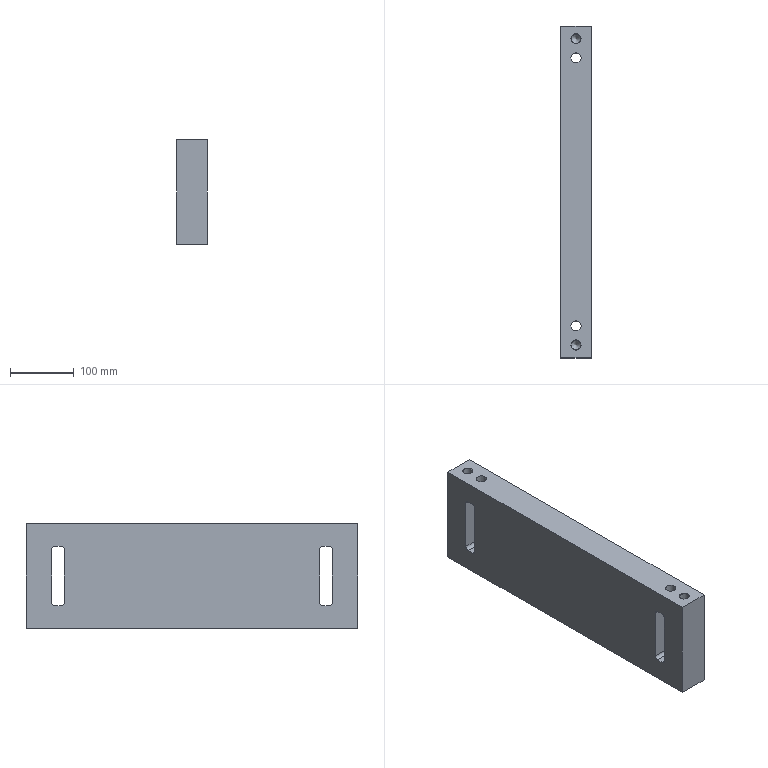Part | NX | features B2-1 2 | 1 solid | 42 faces | box 48 x 520 x 163 mm | volume 3822471 mm3 | plane 18 | cylinder 16 | cone 8 | commonest cylinder face diameters 10 x8 14.506 x4 16 x4
STEP:
#1=CARTESIAN_POINT('',(2312.849,-654.122,698.716));
#2=VERTEX_POINT('',#1);
#3=CARTESIAN_POINT('',(2312.849,-644.122,698.716));
#4=VERTEX_POINT('',#3);
#5=CARTESIAN_POINT('',(2319.094,-649.122,698.716));
#6=DIRECTION('',(0.,0.,1.));
#7=DIRECTION('',(1.,0.,0.));
#8=AXIS2_PLACEMENT_3D('',#5,#6,#7);
#9=CIRCLE('',#8,8.);
#10=EDGE_CURVE('',#2,#4,#9,.F.);
#11=ORIENTED_EDGE('',*,*,#10,.T.);
#12=CARTESIAN_POINT('',(2325.339,-644.122,698.716));
#13=VERTEX_POINT('',#12);
#14=CARTESIAN_POINT('',(2312.849,-644.122,698.716));
#15=CARTESIAN_POINT('',(2313.613,-643.167,698.716));
#16=CARTESIAN_POINT('',(2315.499,-641.68,698.187));
#17=CARTESIAN_POINT('',(2319.097,-640.842,697.481));
#18=CARTESIAN_POINT('',(2322.692,-641.683,698.188));
#19=CARTESIAN_POINT('',(2324.574,-643.166,698.716));
#20=CARTESIAN_POINT('',(2325.339,-644.122,698.716));
#21=B_SPLINE_CURVE_WITH_KNOTS('',3,(#14,#15,#16,#17,#18,#19,#20),.UNSPECIFIED.,.F.,.F.,(4,1,1,1,4),(0.,0.003599,0.007198,0.0108,0.0144),.UNSPECIFIED.);
#22=EDGE_CURVE('',#4,#13,#21,.T.);
#23=ORIENTED_EDGE('',*,*,#22,.T.);
#24=CARTESIAN_POINT('',(2325.339,-654.122,698.716));
#25=VERTEX_POINT('',#24);
#26=CARTESIAN_POINT('',(2319.094,-649.122,698.716));
#27=DIRECTION('',(0.,0.,1.));
#28=DIRECTION('',(1.,0.,0.));
#29=AXIS2_PLACEMENT_3D('',#26,#27,#28);
#30=CIRCLE('',#29,8.);
#31=EDGE_CURVE('',#13,#25,#30,.F.);
#32=ORIENTED_EDGE('',*,*,#31,.T.);
#33=CARTESIAN_POINT('',(2325.339,-654.122,698.716));
#34=CARTESIAN_POINT('',(2324.574,-655.077,698.716));
#35=CARTESIAN_POINT('',(2322.689,-656.564,698.187));
#36=CARTESIAN_POINT('',(2319.091,-657.402,697.481));
#37=CARTESIAN_POINT('',(2315.496,-656.562,698.188));
#38=CARTESIAN_POINT('',(2313.614,-655.078,698.716));
#39=CARTESIAN_POINT('',(2312.849,-654.122,698.716));
#40=B_SPLINE_CURVE_WITH_KNOTS('',3,(#33,#34,#35,#36,#37,#38,#39),.UNSPECIFIED.,.F.,.F.,(4,1,1,1,4),(0.,0.003599,0.007198,0.0108,0.0144),.UNSPECIFIED.);
#41=EDGE_CURVE('',#25,#2,#40,.T.);
#42=ORIENTED_EDGE('',*,*,#41,.T.);
#43=EDGE_LOOP('',(#11,#23,#32,#42));
#44=FACE_BOUND('',#43,.T.);
#45=CARTESIAN_POINT('',(2311.094,-649.122,733.716));
#46=VERTEX_POINT('',#45);
#47=CARTESIAN_POINT('',(2319.094,-649.122,733.716));
#48=DIRECTION('',(0.,0.,-1.));
#49=DIRECTION('',(-1.,0.,0.));
#50=AXIS2_PLACEMENT_3D('',#47,#48,#49);
#51=CIRCLE('',#50,8.);
#52=EDGE_CURVE('',#46,#46,#51,.T.);
#53=ORIENTED_EDGE('',*,*,#52,.F.);
#54=EDGE_LOOP('',(#53));
#55=FACE_BOUND('',#54,.T.);
#56=CARTESIAN_POINT('',(2319.094,-649.122,633.716));
#57=DIRECTION('',(0.,0.,1.));
#58=DIRECTION('',(1.,0.,0.));
#59=AXIS2_PLACEMENT_3D('',#56,#57,#58);
#60=CYLINDRICAL_SURFACE('',#59,8.);
#61=ADVANCED_FACE('',(#44,#55),#60,.F.);
#62=CARTESIAN_POINT('',(2312.849,-1074.122,698.716));
#63=VERTEX_POINT('',#62);
#64=CARTESIAN_POINT('',(2312.849,-1064.122,698.716));
#65=VERTEX_POINT('',#64);
#66=CARTESIAN_POINT('',(2319.094,-1069.122,698.716));
#67=DIRECTION('',(0.,0.,1.));
#68=DIRECTION('',(1.,0.,0.));
#69=AXIS2_PLACEMENT_3D('',#66,#67,#68);
#70=CIRCLE('',#69,8.);
#71=EDGE_CURVE('',#63,#65,#70,.F.);
#72=ORIENTED_EDGE('',*,*,#71,.T.);
#73=CARTESIAN_POINT('',(2325.339,-1064.122,698.716));
#74=VERTEX_POINT('',#73);
#75=CARTESIAN_POINT('',(2312.849,-1064.122,698.716));
#76=CARTESIAN_POINT('',(2313.613,-1063.167,698.716));
#77=CARTESIAN_POINT('',(2315.499,-1061.68,698.187));
#78=CARTESIAN_POINT('',(2319.097,-1060.842,697.481));
#79=CARTESIAN_POINT('',(2322.692,-1061.683,698.188));
#80=CARTESIAN_POINT('',(2324.574,-1063.166,698.716));
#81=CARTESIAN_POINT('',(2325.339,-1064.122,698.716));
#82=B_SPLINE_CURVE_WITH_KNOTS('',3,(#75,#76,#77,#78,#79,#80,#81),.UNSPECIFIED.,.F.,.F.,(4,1,1,1,4),(0.,0.003599,0.007198,0.0108,0.0144),.UNSPECIFIED.);
#83=EDGE_CURVE('',#65,#74,#82,.T.);
#84=ORIENTED_EDGE('',*,*,#83,.T.);
#85=CARTESIAN_POINT('',(2325.339,-1074.122,698.716));
#86=VERTEX_POINT('',#85);
#87=CARTESIAN_POINT('',(2319.094,-1069.122,698.716));
#88=DIRECTION('',(0.,0.,1.));
#89=DIRECTION('',(1.,0.,0.));
#90=AXIS2_PLACEMENT_3D('',#87,#88,#89);
#91=CIRCLE('',#90,8.);
#92=EDGE_CURVE('',#74,#86,#91,.F.);
#93=ORIENTED_EDGE('',*,*,#92,.T.);
#94=CARTESIAN_POINT('',(2325.339,-1074.122,698.716));
#95=CARTESIAN_POINT('',(2324.574,-1075.077,698.716));
#96=CARTESIAN_POINT('',(2322.689,-1076.564,698.187));
#97=CARTESIAN_POINT('',(2319.091,-1077.402,697.481));
#98=CARTESIAN_POINT('',(2315.496,-1076.562,698.188));
#99=CARTESIAN_POINT('',(2313.614,-1075.078,698.716));
#100=CARTESIAN_POINT('',(2312.849,-1074.122,698.716));
#101=B_SPLINE_CURVE_WITH_KNOTS('',3,(#94,#95,#96,#97,#98,#99,#100),.UNSPECIFIED.,.F.,.F.,(4,1,1,1,4),(0.,0.003599,0.007198,0.0108,0.0144),.UNSPECIFIED.);
#102=EDGE_CURVE('',#86,#63,#101,.T.);
#103=ORIENTED_EDGE('',*,*,#102,.T.);
#104=EDGE_LOOP('',(#72,#84,#93,#103));
#105=FACE_BOUND('',#104,.T.);
#106=CARTESIAN_POINT('',(2311.094,-1069.122,733.716));
#107=VERTEX_POINT('',#106);
#108=CARTESIAN_POINT('',(2319.094,-1069.122,733.716));
#109=DIRECTION('',(0.,0.,-1.));
#110=DIRECTION('',(-1.,0.,0.));
#111=AXIS2_PLACEMENT_3D('',#108,#109,#110);
#112=CIRCLE('',#111,8.);
#113=EDGE_CURVE('',#107,#107,#112,.T.);
#114=ORIENTED_EDGE('',*,*,#113,.F.);
#115=EDGE_LOOP('',(#114));
#116=FACE_BOUND('',#115,.T.);
#117=CARTESIAN_POINT('',(2319.094,-1069.122,633.716));
#118=DIRECTION('',(0.,0.,1.));
#119=DIRECTION('',(1.,0.,0.));
#120=AXIS2_PLACEMENT_3D('',#117,#118,#119);
#121=CYLINDRICAL_SURFACE('',#120,8.);
#122=ADVANCED_FACE('',(#105,#116),#121,.F.);
#123=CARTESIAN_POINT('',(2295.094,-639.122,610.716));
#124=VERTEX_POINT('',#123);
#125=CARTESIAN_POINT('',(2295.094,-639.122,693.716));
#126=VERTEX_POINT('',#125);
#127=CARTESIAN_POINT('',(2295.094,-639.122,600.716));
#128=DIRECTION('',(0.,0.,1.));
#129=VECTOR('',#128,1000.);
#130=LINE('',#127,#129);
#131=EDGE_CURVE('',#124,#126,#130,.T.);
#132=ORIENTED_EDGE('',*,*,#131,.T.);
#133=CARTESIAN_POINT('',(2295.094,-644.122,698.716));
#134=VERTEX_POINT('',#133);
#135=CARTESIAN_POINT('',(2295.094,-644.122,693.716));
#136=DIRECTION('',(1.,0.,0.));
#137=DIRECTION('',(0.,0.,-1.));
#138=AXIS2_PLACEMENT_3D('',#135,#136,#137);
#139=CIRCLE('',#138,5.);
#140=EDGE_CURVE('',#126,#134,#139,.T.);
#141=ORIENTED_EDGE('',*,*,#140,.T.);
#142=CARTESIAN_POINT('',(2295.094,-654.122,698.716));
#143=VERTEX_POINT('',#142);
#144=CARTESIAN_POINT('',(2295.094,-599.122,698.716));
#145=DIRECTION('',(0.,-1.,0.));
#146=VECTOR('',#145,1000.);
#147=LINE('',#144,#146);
#148=EDGE_CURVE('',#134,#143,#147,.T.);
#149=ORIENTED_EDGE('',*,*,#148,.T.);
#150=CARTESIAN_POINT('',(2295.094,-659.122,693.716));
#151=VERTEX_POINT('',#150);
#152=CARTESIAN_POINT('',(2295.094,-654.122,693.716));
#153=DIRECTION('',(1.,0.,0.));
#154=DIRECTION('',(0.,0.,-1.));
#155=AXIS2_PLACEMENT_3D('',#152,#153,#154);
#156=CIRCLE('',#155,5.);
#157=EDGE_CURVE('',#143,#151,#156,.T.);
#158=ORIENTED_EDGE('',*,*,#157,.T.);
#159=CARTESIAN_POINT('',(2295.094,-659.122,610.716));
#160=VERTEX_POINT('',#159);
#161=CARTESIAN_POINT('',(2295.094,-659.122,600.716));
#162=DIRECTION('',(0.,0.,-1.));
#163=VECTOR('',#162,1000.);
#164=LINE('',#161,#163);
#165=EDGE_CURVE('',#151,#160,#164,.T.);
#166=ORIENTED_EDGE('',*,*,#165,.T.);
#167=CARTESIAN_POINT('',(2295.094,-654.122,605.716));
#168=VERTEX_POINT('',#167);
#169=CARTESIAN_POINT('',(2295.094,-654.122,610.716));
#170=DIRECTION('',(1.,0.,0.));
#171=DIRECTION('',(0.,0.,-1.));
#172=AXIS2_PLACEMENT_3D('',#169,#170,#171);
#173=CIRCLE('',#172,5.);
#174=EDGE_CURVE('',#160,#168,#173,.T.);
#175=ORIENTED_EDGE('',*,*,#174,.T.);
#176=CARTESIAN_POINT('',(2295.094,-644.122,605.716));
#177=VERTEX_POINT('',#176);
#178=CARTESIAN_POINT('',(2295.094,-599.122,605.716));
#179=DIRECTION('',(0.,1.,0.));
#180=VECTOR('',#179,1000.);
#181=LINE('',#178,#180);
#182=EDGE_CURVE('',#168,#177,#181,.T.);
#183=ORIENTED_EDGE('',*,*,#182,.T.);
#184=CARTESIAN_POINT('',(2295.094,-644.122,610.716));
#185=DIRECTION('',(1.,0.,0.));
#186=DIRECTION('',(0.,0.,-1.));
#187=AXIS2_PLACEMENT_3D('',#184,#185,#186);
#188=CIRCLE('',#187,5.);
#189=EDGE_CURVE('',#177,#124,#188,.T.);
#190=ORIENTED_EDGE('',*,*,#189,.T.);
#191=EDGE_LOOP('',(#132,#141,#149,#158,#166,#175,#183,#190));
#192=FACE_BOUND('',#191,.T.);
#193=CARTESIAN_POINT('',(2295.094,-1059.122,610.716));
#194=VERTEX_POINT('',#193);
#195=CARTESIAN_POINT('',(2295.094,-1059.122,693.716));
#196=VERTEX_POINT('',#195);
#197=CARTESIAN_POINT('',(2295.094,-1059.122,600.716));
#198=DIRECTION('',(0.,0.,1.));
#199=VECTOR('',#198,1000.);
#200=LINE('',#197,#199);
#201=EDGE_CURVE('',#194,#196,#200,.T.);
#202=ORIENTED_EDGE('',*,*,#201,.T.);
#203=CARTESIAN_POINT('',(2295.094,-1064.122,698.716));
#204=VERTEX_POINT('',#203);
#205=CARTESIAN_POINT('',(2295.094,-1064.122,693.716));
#206=DIRECTION('',(1.,0.,0.));
#207=DIRECTION('',(0.,0.,-1.));
#208=AXIS2_PLACEMENT_3D('',#205,#206,#207);
#209=CIRCLE('',#208,5.);
#210=EDGE_CURVE('',#196,#204,#209,.T.);
#211=ORIENTED_EDGE('',*,*,#210,.T.);
#212=CARTESIAN_POINT('',(2295.094,-1074.122,698.716));
#213=VERTEX_POINT('',#212);
#214=CARTESIAN_POINT('',(2295.094,-599.122,698.716));
#215=DIRECTION('',(0.,-1.,0.));
#216=VECTOR('',#215,1000.);
#217=LINE('',#214,#216);
#218=EDGE_CURVE('',#204,#213,#217,.T.);
#219=ORIENTED_EDGE('',*,*,#218,.T.);
#220=CARTESIAN_POINT('',(2295.094,-1079.122,693.716));
#221=VERTEX_POINT('',#220);
#222=CARTESIAN_POINT('',(2295.094,-1074.122,693.716));
#223=DIRECTION('',(1.,0.,0.));
#224=DIRECTION('',(0.,0.,-1.));
#225=AXIS2_PLACEMENT_3D('',#222,#223,#224);
#226=CIRCLE('',#225,5.);
#227=EDGE_CURVE('',#213,#221,#226,.T.);
#228=ORIENTED_EDGE('',*,*,#227,.T.);
#229=CARTESIAN_POINT('',(2295.094,-1079.122,610.716));
#230=VERTEX_POINT('',#229);
#231=CARTESIAN_POINT('',(2295.094,-1079.122,600.716));
#232=DIRECTION('',(0.,0.,-1.));
#233=VECTOR('',#232,1000.);
#234=LINE('',#231,#233);
#235=EDGE_CURVE('',#221,#230,#234,.T.);
#236=ORIENTED_EDGE('',*,*,#235,.T.);
#237=CARTESIAN_POINT('',(2295.094,-1074.122,605.716));
#238=VERTEX_POINT('',#237);
#239=CARTESIAN_POINT('',(2295.094,-1074.122,610.716));
#240=DIRECTION('',(1.,0.,0.));
#241=DIRECTION('',(0.,0.,-1.));
#242=AXIS2_PLACEMENT_3D('',#239,#240,#241);
#243=CIRCLE('',#242,5.);
#244=EDGE_CURVE('',#230,#238,#243,.T.);
#245=ORIENTED_EDGE('',*,*,#244,.T.);
#246=CARTESIAN_POINT('',(2295.094,-1064.122,605.716));
#247=VERTEX_POINT('',#246);
#248=CARTESIAN_POINT('',(2295.094,-599.122,605.716));
#249=DIRECTION('',(0.,1.,0.));
#250=VECTOR('',#249,1000.);
#251=LINE('',#248,#250);
#252=EDGE_CURVE('',#238,#247,#251,.T.);
#253=ORIENTED_EDGE('',*,*,#252,.T.);
#254=CARTESIAN_POINT('',(2295.094,-1064.122,610.716));
#255=DIRECTION('',(1.,0.,0.));
#256=DIRECTION('',(0.,0.,-1.));
#257=AXIS2_PLACEMENT_3D('',#254,#255,#256);
#258=CIRCLE('',#257,5.);
#259=EDGE_CURVE('',#247,#194,#258,.T.);
#260=ORIENTED_EDGE('',*,*,#259,.T.);
#261=EDGE_LOOP('',(#202,#211,#219,#228,#236,#245,#253,#260));
#262=FACE_BOUND('',#261,.T.);
#263=CARTESIAN_POINT('',(2295.094,-599.122,733.716));
#264=VERTEX_POINT('',#263);
#265=CARTESIAN_POINT('',(2295.094,-1119.122,733.716));
#266=VERTEX_POINT('',#265);
#267=CARTESIAN_POINT('',(2295.094,-599.122,733.716));
#268=DIRECTION('',(0.,-1.,0.));
#269=VECTOR('',#268,1000.);
#270=LINE('',#267,#269);
#271=EDGE_CURVE('',#264,#266,#270,.T.);
#272=ORIENTED_EDGE('',*,*,#271,.F.);
#273=CARTESIAN_POINT('',(2295.094,-599.122,570.716));
#274=VERTEX_POINT('',#273);
#275=CARTESIAN_POINT('',(2295.094,-599.122,600.716));
#276=DIRECTION('',(0.,0.,1.));
#277=VECTOR('',#276,1000.);
#278=LINE('',#275,#277);
#279=EDGE_CURVE('',#274,#264,#278,.T.);
#280=ORIENTED_EDGE('',*,*,#279,.F.);
#281=CARTESIAN_POINT('',(2295.094,-1119.122,570.716));
#282=VERTEX_POINT('',#281);
#283=CARTESIAN_POINT('',(2295.094,-599.122,570.716));
#284=DIRECTION('',(0.,-1.,0.));
#285=VECTOR('',#284,1000.);
#286=LINE('',#283,#285);
#287=EDGE_CURVE('',#274,#282,#286,.T.);
#288=ORIENTED_EDGE('',*,*,#287,.T.);
#289=CARTESIAN_POINT('',(2295.094,-1119.122,600.716));
#290=DIRECTION('',(0.,0.,1.));
#291=VECTOR('',#290,1000.);
#292=LINE('',#289,#291);
#293=EDGE_CURVE('',#282,#266,#292,.T.);
#294=ORIENTED_EDGE('',*,*,#293,.T.);
#295=EDGE_LOOP('',(#272,#280,#288,#294));
#296=FACE_BOUND('',#295,.T.);
#297=CARTESIAN_POINT('',(2295.094,-599.122,600.716));
#298=DIRECTION('',(1.,0.,0.));
#299=DIRECTION('',(0.,0.,1.));
#300=AXIS2_PLACEMENT_3D('',#297,#298,#299);
#301=PLANE('',#300);
#302=ADVANCED_FACE('',(#192,#262,#296),#301,.F.);
#303=CARTESIAN_POINT('',(2311.094,-649.122,570.716));
#304=VERTEX_POINT('',#303);
#305=CARTESIAN_POINT('',(2319.094,-649.122,570.716));
#306=DIRECTION('',(0.,0.,-1.));
#307=DIRECTION('',(-1.,0.,0.));
#308=AXIS2_PLACEMENT_3D('',#305,#306,#307);
#309=CIRCLE('',#308,8.);
#310=EDGE_CURVE('',#304,#304,#309,.T.);
#311=ORIENTED_EDGE('',*,*,#310,.F.);
#312=EDGE_LOOP('',(#311));
#313=FACE_BOUND('',#312,.T.);
#314=CARTESIAN_POINT('',(2311.094,-1069.122,570.716));
#315=VERTEX_POINT('',#314);
#316=CARTESIAN_POINT('',(2319.094,-1069.122,570.716));
#317=DIRECTION('',(0.,0.,-1.));
#318=DIRECTION('',(-1.,0.,0.));
#319=AXIS2_PLACEMENT_3D('',#316,#317,#318);
#320=CIRCLE('',#319,8.);
#321=EDGE_CURVE('',#315,#315,#320,.T.);
#322=ORIENTED_EDGE('',*,*,#321,.F.);
#323=EDGE_LOOP('',(#322));
#324=FACE_BOUND('',#323,.T.);
#325=CARTESIAN_POINT('',(2311.094,-679.122,570.716));
#326=VERTEX_POINT('',#325);
#327=CARTESIAN_POINT('',(2319.094,-679.122,570.716));
#328=DIRECTION('',(0.,0.,-1.));
#329=DIRECTION('',(-1.,0.,0.));
#330=AXIS2_PLACEMENT_3D('',#327,#328,#329);
#331=CIRCLE('',#330,8.);
#332=EDGE_CURVE('',#326,#326,#331,.T.);
#333=ORIENTED_EDGE('',*,*,#332,.F.);
#334=EDGE_LOOP('',(#333));
#335=FACE_BOUND('',#334,.T.);
#336=CARTESIAN_POINT('',(2311.094,-1039.122,570.716));
#337=VERTEX_POINT('',#336);
#338=CARTESIAN_POINT('',(2319.094,-1039.122,570.716));
#339=DIRECTION('',(0.,0.,-1.));
#340=DIRECTION('',(-1.,0.,0.));
#341=AXIS2_PLACEMENT_3D('',#338,#339,#340);
#342=CIRCLE('',#341,8.);
#343=EDGE_CURVE('',#337,#337,#342,.T.);
#344=ORIENTED_EDGE('',*,*,#343,.F.);
#345=EDGE_LOOP('',(#344));
#346=FACE_BOUND('',#345,.T.);
#347=CARTESIAN_POINT('',(2343.094,-599.122,570.716));
#348=VERTEX_POINT('',#347);
#349=CARTESIAN_POINT('',(2343.094,-1119.122,570.716));
#350=VERTEX_POINT('',#349);
#351=CARTESIAN_POINT('',(2343.094,0.,570.716));
#352=DIRECTION('',(0.,-1.,0.));
#353=VECTOR('',#352,1000.);
#354=LINE('',#351,#353);
#355=EDGE_CURVE('',#348,#350,#354,.T.);
#356=ORIENTED_EDGE('',*,*,#355,.T.);
#357=CARTESIAN_POINT('',(2295.094,-1119.122,570.716));
#358=DIRECTION('',(1.,0.,0.));
#359=VECTOR('',#358,1000.);
#360=LINE('',#357,#359);
#361=EDGE_CURVE('',#282,#350,#360,.T.);
#362=ORIENTED_EDGE('',*,*,#361,.F.);
#363=ORIENTED_EDGE('',*,*,#287,.F.);
#364=CARTESIAN_POINT('',(4420.094,-599.122,570.716));
#365=DIRECTION('',(-1.,0.,0.));
#366=VECTOR('',#365,1000.);
#367=LINE('',#364,#366);
#368=EDGE_CURVE('',#348,#274,#367,.T.);
#369=ORIENTED_EDGE('',*,*,#368,.F.);
#370=EDGE_LOOP('',(#356,#362,#363,#369));
#371=FACE_BOUND('',#370,.T.);
#372=CARTESIAN_POINT('',(6675.188,0.,570.716));
#373=DIRECTION('',(0.,0.,-1.));
#374=DIRECTION('',(1.,0.,0.));
#375=AXIS2_PLACEMENT_3D('',#372,#373,#374);
#376=PLANE('',#375);
#377=ADVANCED_FACE('',(#313,#324,#335,#346,#371),#376,.T.);
#378=ORIENTED_EDGE('',*,*,#52,.T.);
#379=EDGE_LOOP('',(#378));
#380=FACE_BOUND('',#379,.T.);
#381=ORIENTED_EDGE('',*,*,#113,.T.);
#382=EDGE_LOOP('',(#381));
#383=FACE_BOUND('',#382,.T.);
#384=CARTESIAN_POINT('',(2327.094,-619.122,733.716));
#385=VERTEX_POINT('',#384);
#386=CARTESIAN_POINT('',(2319.094,-619.122,733.716));
#387=DIRECTION('',(0.,0.,1.));
#388=DIRECTION('',(1.,0.,0.));
#389=AXIS2_PLACEMENT_3D('',#386,#387,#388);
#390=CIRCLE('',#389,8.);
#391=EDGE_CURVE('',#385,#385,#390,.T.);
#392=ORIENTED_EDGE('',*,*,#391,.F.);
#393=EDGE_LOOP('',(#392));
#394=FACE_BOUND('',#393,.T.);
#395=CARTESIAN_POINT('',(2327.094,-1099.122,733.716));
#396=VERTEX_POINT('',#395);
#397=CARTESIAN_POINT('',(2319.094,-1099.122,733.716));
#398=DIRECTION('',(0.,0.,1.));
#399=DIRECTION('',(1.,0.,0.));
#400=AXIS2_PLACEMENT_3D('',#397,#398,#399);
#401=CIRCLE('',#400,8.);
#402=EDGE_CURVE('',#396,#396,#401,.T.);
#403=ORIENTED_EDGE('',*,*,#402,.F.);
#404=EDGE_LOOP('',(#403));
#405=FACE_BOUND('',#404,.T.);
#406=CARTESIAN_POINT('',(2343.094,-599.122,733.716));
#407=VERTEX_POINT('',#406);
#408=CARTESIAN_POINT('',(4420.094,-599.122,733.716));
#409=DIRECTION('',(-1.,0.,0.));
#410=VECTOR('',#409,1000.);
#411=LINE('',#408,#410);
#412=EDGE_CURVE('',#407,#264,#411,.T.);
#413=ORIENTED_EDGE('',*,*,#412,.T.);
#414=ORIENTED_EDGE('',*,*,#271,.T.);
#415=CARTESIAN_POINT('',(2343.094,-1119.122,733.716));
#416=VERTEX_POINT('',#415);
#417=CARTESIAN_POINT('',(2295.094,-1119.122,733.716));
#418=DIRECTION('',(1.,0.,0.));
#419=VECTOR('',#418,1000.);
#420=LINE('',#417,#419);
#421=EDGE_CURVE('',#266,#416,#420,.T.);
#422=ORIENTED_EDGE('',*,*,#421,.T.);
#423=CARTESIAN_POINT('',(2343.094,-859.122,733.716));
#424=DIRECTION('',(0.,1.,0.));
#425=VECTOR('',#424,1000.);
#426=LINE('',#423,#425);
#427=EDGE_CURVE('',#416,#407,#426,.T.);
#428=ORIENTED_EDGE('',*,*,#427,.T.);
#429=EDGE_LOOP('',(#413,#414,#422,#428));
#430=FACE_BOUND('',#429,.T.);
#431=CARTESIAN_POINT('',(6675.188,0.,733.716));
#432=DIRECTION('',(0.,0.,-1.));
#433=DIRECTION('',(1.,0.,0.));
#434=AXIS2_PLACEMENT_3D('',#431,#432,#433);
#435=PLANE('',#434);
#436=ADVANCED_FACE('',(#380,#383,#394,#405,#430),#435,.F.);
#437=ORIENTED_EDGE('',*,*,#421,.F.);
#438=ORIENTED_EDGE('',*,*,#293,.F.);
#439=ORIENTED_EDGE('',*,*,#361,.T.);
#440=CARTESIAN_POINT('',(2343.094,-1119.122,600.716));
#441=DIRECTION('',(0.,0.,-1.));
#442=VECTOR('',#441,1000.);
#443=LINE('',#440,#442);
#444=EDGE_CURVE('',#416,#350,#443,.T.);
#445=ORIENTED_EDGE('',*,*,#444,.F.);
#446=EDGE_LOOP('',(#437,#438,#439,#445));
#447=FACE_BOUND('',#446,.T.);
#448=CARTESIAN_POINT('',(2295.094,-1119.122,600.716));
#449=DIRECTION('',(0.,1.,0.));
#450=DIRECTION('',(1.,0.,0.));
#451=AXIS2_PLACEMENT_3D('',#448,#449,#450);
#452=PLANE('',#451);
#453=ADVANCED_FACE('',(#447),#452,.F.);
#454=ORIENTED_EDGE('',*,*,#368,.T.);
#455=ORIENTED_EDGE('',*,*,#279,.T.);
#456=ORIENTED_EDGE('',*,*,#412,.F.);
#457=CARTESIAN_POINT('',(2343.094,-599.122,600.716));
#458=DIRECTION('',(0.,0.,1.));
#459=VECTOR('',#458,1000.);
#460=LINE('',#457,#459);
#461=EDGE_CURVE('',#348,#407,#460,.T.);
#462=ORIENTED_EDGE('',*,*,#461,.F.);
#463=EDGE_LOOP('',(#454,#455,#456,#462));
#464=FACE_BOUND('',#463,.T.);
#465=CARTESIAN_POINT('',(4420.094,-599.122,600.716));
#466=DIRECTION('',(0.,-1.,0.));
#467=DIRECTION('',(0.,0.,-1.));
#468=AXIS2_PLACEMENT_3D('',#465,#466,#467);
#469=PLANE('',#468);
#470=ADVANCED_FACE('',(#464),#469,.F.);
#471=CARTESIAN_POINT('',(2343.094,-654.122,698.716));
#472=VERTEX_POINT('',#471);
#473=CARTESIAN_POINT('',(2343.094,-644.122,698.716));
#474=VERTEX_POINT('',#473);
#475=CARTESIAN_POINT('',(2343.094,-859.122,698.716));
#476=DIRECTION('',(0.,1.,0.));
#477=VECTOR('',#476,1000.);
#478=LINE('',#475,#477);
#479=EDGE_CURVE('',#472,#474,#478,.T.);
#480=ORIENTED_EDGE('',*,*,#479,.T.);
#481=CARTESIAN_POINT('',(2343.094,-639.122,693.716));
#482=VERTEX_POINT('',#481);
#483=CARTESIAN_POINT('',(2343.094,-644.122,693.716));
#484=DIRECTION('',(-1.,0.,0.));
#485=DIRECTION('',(0.,0.,1.));
#486=AXIS2_PLACEMENT_3D('',#483,#484,#485);
#487=CIRCLE('',#486,5.);
#488=EDGE_CURVE('',#474,#482,#487,.T.);
#489=ORIENTED_EDGE('',*,*,#488,.T.);
#490=CARTESIAN_POINT('',(2343.094,-639.122,610.716));
#491=VERTEX_POINT('',#490);
#492=CARTESIAN_POINT('',(2343.094,-639.122,667.216));
#493=DIRECTION('',(0.,0.,-1.));
#494=VECTOR('',#493,1000.);
#495=LINE('',#492,#494);
#496=EDGE_CURVE('',#482,#491,#495,.T.);
#497=ORIENTED_EDGE('',*,*,#496,.T.);
#498=CARTESIAN_POINT('',(2343.094,-644.122,605.716));
#499=VERTEX_POINT('',#498);
#500=CARTESIAN_POINT('',(2343.094,-644.122,610.716));
#501=DIRECTION('',(-1.,0.,0.));
#502=DIRECTION('',(0.,0.,1.));
#503=AXIS2_PLACEMENT_3D('',#500,#501,#502);
#504=CIRCLE('',#503,5.);
#505=EDGE_CURVE('',#491,#499,#504,.T.);
#506=ORIENTED_EDGE('',*,*,#505,.T.);
#507=CARTESIAN_POINT('',(2343.094,-654.122,605.716));
#508=VERTEX_POINT('',#507);
#509=CARTESIAN_POINT('',(2343.094,-859.122,605.716));
#510=DIRECTION('',(0.,-1.,0.));
#511=VECTOR('',#510,1000.);
#512=LINE('',#509,#511);
#513=EDGE_CURVE('',#499,#508,#512,.T.);
#514=ORIENTED_EDGE('',*,*,#513,.T.);
#515=CARTESIAN_POINT('',(2343.094,-659.122,610.716));
#516=VERTEX_POINT('',#515);
#517=CARTESIAN_POINT('',(2343.094,-654.122,610.716));
#518=DIRECTION('',(-1.,0.,0.));
#519=DIRECTION('',(0.,0.,1.));
#520=AXIS2_PLACEMENT_3D('',#517,#518,#519);
#521=CIRCLE('',#520,5.);
#522=EDGE_CURVE('',#508,#516,#521,.T.);
#523=ORIENTED_EDGE('',*,*,#522,.T.);
#524=CARTESIAN_POINT('',(2343.094,-659.122,693.716));
#525=VERTEX_POINT('',#524);
#526=CARTESIAN_POINT('',(2343.094,-659.122,667.216));
#527=DIRECTION('',(0.,0.,1.));
#528=VECTOR('',#527,1000.);
#529=LINE('',#526,#528);
#530=EDGE_CURVE('',#516,#525,#529,.T.);
#531=ORIENTED_EDGE('',*,*,#530,.T.);
#532=CARTESIAN_POINT('',(2343.094,-654.122,693.716));
#533=DIRECTION('',(-1.,0.,0.));
#534=DIRECTION('',(0.,0.,1.));
#535=AXIS2_PLACEMENT_3D('',#532,#533,#534);
#536=CIRCLE('',#535,5.);
#537=EDGE_CURVE('',#525,#472,#536,.T.);
#538=ORIENTED_EDGE('',*,*,#537,.T.);
#539=EDGE_LOOP('',(#480,#489,#497,#506,#514,#523,#531,#538));
#540=FACE_BOUND('',#539,.T.);
#541=CARTESIAN_POINT('',(2343.094,-1074.122,698.716));
#542=VERTEX_POINT('',#541);
#543=CARTESIAN_POINT('',(2343.094,-1064.122,698.716));
#544=VERTEX_POINT('',#543);
#545=CARTESIAN_POINT('',(2343.094,-859.122,698.716));
#546=DIRECTION('',(0.,1.,0.));
#547=VECTOR('',#546,1000.);
#548=LINE('',#545,#547);
#549=EDGE_CURVE('',#542,#544,#548,.T.);
#550=ORIENTED_EDGE('',*,*,#549,.T.);
#551=CARTESIAN_POINT('',(2343.094,-1059.122,693.716));
#552=VERTEX_POINT('',#551);
#553=CARTESIAN_POINT('',(2343.094,-1064.122,693.716));
#554=DIRECTION('',(-1.,0.,0.));
#555=DIRECTION('',(0.,0.,1.));
#556=AXIS2_PLACEMENT_3D('',#553,#554,#555);
#557=CIRCLE('',#556,5.);
#558=EDGE_CURVE('',#544,#552,#557,.T.);
#559=ORIENTED_EDGE('',*,*,#558,.T.);
#560=CARTESIAN_POINT('',(2343.094,-1059.122,610.716));
#561=VERTEX_POINT('',#560);
#562=CARTESIAN_POINT('',(2343.094,-1059.122,667.216));
#563=DIRECTION('',(0.,0.,-1.));
#564=VECTOR('',#563,1000.);
#565=LINE('',#562,#564);
#566=EDGE_CURVE('',#552,#561,#565,.T.);
#567=ORIENTED_EDGE('',*,*,#566,.T.);
#568=CARTESIAN_POINT('',(2343.094,-1064.122,605.716));
#569=VERTEX_POINT('',#568);
#570=CARTESIAN_POINT('',(2343.094,-1064.122,610.716));
#571=DIRECTION('',(-1.,0.,0.));
#572=DIRECTION('',(0.,0.,1.));
#573=AXIS2_PLACEMENT_3D('',#570,#571,#572);
#574=CIRCLE('',#573,5.);
#575=EDGE_CURVE('',#561,#569,#574,.T.);
#576=ORIENTED_EDGE('',*,*,#575,.T.);
#577=CARTESIAN_POINT('',(2343.094,-1074.122,605.716));
#578=VERTEX_POINT('',#577);
#579=CARTESIAN_POINT('',(2343.094,-859.122,605.716));
#580=DIRECTION('',(0.,-1.,0.));
#581=VECTOR('',#580,1000.);
#582=LINE('',#579,#581);
#583=EDGE_CURVE('',#569,#578,#582,.T.);
#584=ORIENTED_EDGE('',*,*,#583,.T.);
#585=CARTESIAN_POINT('',(2343.094,-1079.122,610.716));
#586=VERTEX_POINT('',#585);
#587=CARTESIAN_POINT('',(2343.094,-1074.122,610.716));
#588=DIRECTION('',(-1.,0.,0.));
#589=DIRECTION('',(0.,0.,1.));
#590=AXIS2_PLACEMENT_3D('',#587,#588,#589);
#591=CIRCLE('',#590,5.);
#592=EDGE_CURVE('',#578,#586,#591,.T.);
#593=ORIENTED_EDGE('',*,*,#592,.T.);
#594=CARTESIAN_POINT('',(2343.094,-1079.122,693.716));
#595=VERTEX_POINT('',#594);
#596=CARTESIAN_POINT('',(2343.094,-1079.122,667.216));
#597=DIRECTION('',(0.,0.,1.));
#598=VECTOR('',#597,1000.);
#599=LINE('',#596,#598);
#600=EDGE_CURVE('',#586,#595,#599,.T.);
#601=ORIENTED_EDGE('',*,*,#600,.T.);
#602=CARTESIAN_POINT('',(2343.094,-1074.122,693.716));
#603=DIRECTION('',(-1.,0.,0.));
#604=DIRECTION('',(0.,0.,1.));
#605=AXIS2_PLACEMENT_3D('',#602,#603,#604);
#606=CIRCLE('',#605,5.);
#607=EDGE_CURVE('',#595,#542,#606,.T.);
#608=ORIENTED_EDGE('',*,*,#607,.T.);
#609=EDGE_LOOP('',(#550,#559,#567,#576,#584,#593,#601,#608));
#610=FACE_BOUND('',#609,.T.);
#611=ORIENTED_EDGE('',*,*,#355,.F.);
#612=ORIENTED_EDGE('',*,*,#461,.T.);
#613=ORIENTED_EDGE('',*,*,#427,.F.);
#614=ORIENTED_EDGE('',*,*,#444,.T.);
#615=EDGE_LOOP('',(#611,#612,#613,#614));
#616=FACE_BOUND('',#615,.T.);
#617=CARTESIAN_POINT('',(2343.094,-859.122,667.216));
#618=DIRECTION('',(-1.,0.,0.));
#619=DIRECTION('',(0.,0.,-1.));
#620=AXIS2_PLACEMENT_3D('',#617,#618,#619);
#621=PLANE('',#620);
#622=ADVANCED_FACE('',(#540,#610,#616),#621,.F.);
#623=CARTESIAN_POINT('',(2311.841,-1039.122,571.463));
#624=VERTEX_POINT('',#623);
#625=CARTESIAN_POINT('',(2319.094,-1039.122,571.463));
#626=DIRECTION('',(0.,0.,-1.));
#627=DIRECTION('',(-1.,0.,0.));
#628=AXIS2_PLACEMENT_3D('',#625,#626,#627);
#629=CIRCLE('',#628,7.253);
#630=EDGE_CURVE('',#624,#624,#629,.F.);
#631=ORIENTED_EDGE('',*,*,#630,.F.);
#632=EDGE_LOOP('',(#631));
#633=FACE_BOUND('',#632,.T.);
#634=CARTESIAN_POINT('',(2311.841,-1039.122,645.713));
#635=VERTEX_POINT('',#634);
#636=CARTESIAN_POINT('',(2319.094,-1039.122,645.713));
#637=DIRECTION('',(0.,0.,-1.));
#638=DIRECTION('',(-1.,0.,0.));
#639=AXIS2_PLACEMENT_3D('',#636,#637,#638);
#640=CIRCLE('',#639,7.253);
#641=EDGE_CURVE('',#635,#635,#640,.F.);
#642=ORIENTED_EDGE('',*,*,#641,.T.);
#643=EDGE_LOOP('',(#642));
#644=FACE_BOUND('',#643,.T.);
#645=CARTESIAN_POINT('',(2319.094,-1039.122,652.966));
#646=DIRECTION('',(0.,0.,-1.));
#647=DIRECTION('',(-1.,0.,0.));
#648=AXIS2_PLACEMENT_3D('',#645,#646,#647);
#649=CYLINDRICAL_SURFACE('',#648,7.253);
#650=ADVANCED_FACE('',(#633,#644),#649,.F.);
#651=CARTESIAN_POINT('',(2319.094,-1039.122,652.966));
#652=VERTEX_POINT('',#651);
#653=VERTEX_LOOP('',#652);
#654=FACE_BOUND('',#653,.T.);
#655=ORIENTED_EDGE('',*,*,#641,.F.);
#656=EDGE_LOOP('',(#655));
#657=FACE_BOUND('',#656,.T.);
#658=CARTESIAN_POINT('',(2319.094,-1039.122,645.716));
#659=DIRECTION('',(0.,0.,-1.));
#660=DIRECTION('',(-1.,0.,0.));
#661=AXIS2_PLACEMENT_3D('',#658,#659,#660);
#662=CONICAL_SURFACE('',#661,7.25,0.7854);
#663=ADVANCED_FACE('',(#654,#657),#662,.F.);
#664=ORIENTED_EDGE('',*,*,#630,.T.);
#665=EDGE_LOOP('',(#664));
#666=FACE_BOUND('',#665,.T.);
#667=ORIENTED_EDGE('',*,*,#343,.T.);
#668=EDGE_LOOP('',(#667));
#669=FACE_BOUND('',#668,.T.);
#670=CARTESIAN_POINT('',(2319.094,-1039.122,570.716));
#671=DIRECTION('',(0.,0.,-1.));
#672=DIRECTION('',(-1.,0.,0.));
#673=AXIS2_PLACEMENT_3D('',#670,#671,#672);
#674=CONICAL_SURFACE('',#673,8.,0.7854);
#675=ADVANCED_FACE('',(#666,#669),#674,.F.);
#676=CARTESIAN_POINT('',(2311.841,-679.122,571.463));
#677=VERTEX_POINT('',#676);
#678=CARTESIAN_POINT('',(2319.094,-679.122,571.463));
#679=DIRECTION('',(0.,0.,-1.));
#680=DIRECTION('',(-1.,0.,0.));
#681=AXIS2_PLACEMENT_3D('',#678,#679,#680);
#682=CIRCLE('',#681,7.253);
#683=EDGE_CURVE('',#677,#677,#682,.F.);
#684=ORIENTED_EDGE('',*,*,#683,.F.);
#685=EDGE_LOOP('',(#684));
#686=FACE_BOUND('',#685,.T.);
#687=CARTESIAN_POINT('',(2311.841,-679.122,645.713));
#688=VERTEX_POINT('',#687);
#689=CARTESIAN_POINT('',(2319.094,-679.122,645.713));
#690=DIRECTION('',(0.,0.,-1.));
#691=DIRECTION('',(-1.,0.,0.));
#692=AXIS2_PLACEMENT_3D('',#689,#690,#691);
#693=CIRCLE('',#692,7.253);
#694=EDGE_CURVE('',#688,#688,#693,.F.);
#695=ORIENTED_EDGE('',*,*,#694,.T.);
#696=EDGE_LOOP('',(#695));
#697=FACE_BOUND('',#696,.T.);
#698=CARTESIAN_POINT('',(2319.094,-679.122,652.966));
#699=DIRECTION('',(0.,0.,-1.));
#700=DIRECTION('',(-1.,0.,0.));
#701=AXIS2_PLACEMENT_3D('',#698,#699,#700);
#702=CYLINDRICAL_SURFACE('',#701,7.253);
#703=ADVANCED_FACE('',(#686,#697),#702,.F.);
#704=CARTESIAN_POINT('',(2319.094,-679.122,652.966));
#705=VERTEX_POINT('',#704);
#706=VERTEX_LOOP('',#705);
#707=FACE_BOUND('',#706,.T.);
#708=ORIENTED_EDGE('',*,*,#694,.F.);
#709=EDGE_LOOP('',(#708));
#710=FACE_BOUND('',#709,.T.);
#711=CARTESIAN_POINT('',(2319.094,-679.122,645.716));
#712=DIRECTION('',(0.,0.,-1.));
#713=DIRECTION('',(-1.,0.,0.));
#714=AXIS2_PLACEMENT_3D('',#711,#712,#713);
#715=CONICAL_SURFACE('',#714,7.25,0.7854);
#716=ADVANCED_FACE('',(#707,#710),#715,.F.);
#717=ORIENTED_EDGE('',*,*,#683,.T.);
#718=EDGE_LOOP('',(#717));
#719=FACE_BOUND('',#718,.T.);
#720=ORIENTED_EDGE('',*,*,#332,.T.);
#721=EDGE_LOOP('',(#720));
#722=FACE_BOUND('',#721,.T.);
#723=CARTESIAN_POINT('',(2319.094,-679.122,570.716));
#724=DIRECTION('',(0.,0.,-1.));
#725=DIRECTION('',(-1.,0.,0.));
#726=AXIS2_PLACEMENT_3D('',#723,#724,#725);
#727=CONICAL_SURFACE('',#726,8.,0.7854);
#728=ADVANCED_FACE('',(#719,#722),#727,.F.);
#729=CARTESIAN_POINT('',(2326.347,-1099.122,732.969));
#730=VERTEX_POINT('',#729);
#731=CARTESIAN_POINT('',(2319.094,-1099.122,732.969));
#732=DIRECTION('',(0.,0.,1.));
#733=DIRECTION('',(1.,0.,0.));
#734=AXIS2_PLACEMENT_3D('',#731,#732,#733);
#735=CIRCLE('',#734,7.253);
#736=EDGE_CURVE('',#730,#730,#735,.F.);
#737=ORIENTED_EDGE('',*,*,#736,.F.);
#738=EDGE_LOOP('',(#737));
#739=FACE_BOUND('',#738,.T.);
#740=CARTESIAN_POINT('',(2326.347,-1099.122,688.719));
#741=VERTEX_POINT('',#740);
#742=CARTESIAN_POINT('',(2319.094,-1099.122,688.719));
#743=DIRECTION('',(0.,0.,1.));
#744=DIRECTION('',(1.,0.,0.));
#745=AXIS2_PLACEMENT_3D('',#742,#743,#744);
#746=CIRCLE('',#745,7.253);
#747=EDGE_CURVE('',#741,#741,#746,.F.);
#748=ORIENTED_EDGE('',*,*,#747,.T.);
#749=EDGE_LOOP('',(#748));
#750=FACE_BOUND('',#749,.T.);
#751=CARTESIAN_POINT('',(2319.094,-1099.122,681.466));
#752=DIRECTION('',(0.,0.,1.));
#753=DIRECTION('',(1.,0.,0.));
#754=AXIS2_PLACEMENT_3D('',#751,#752,#753);
#755=CYLINDRICAL_SURFACE('',#754,7.253);
#756=ADVANCED_FACE('',(#739,#750),#755,.F.);
#757=CARTESIAN_POINT('',(2319.094,-1099.122,681.466));
#758=VERTEX_POINT('',#757);
#759=VERTEX_LOOP('',#758);
#760=FACE_BOUND('',#759,.T.);
#761=ORIENTED_EDGE('',*,*,#747,.F.);
#762=EDGE_LOOP('',(#761));
#763=FACE_BOUND('',#762,.T.);
#764=CARTESIAN_POINT('',(2319.094,-1099.122,688.716));
#765=DIRECTION('',(0.,0.,1.));
#766=DIRECTION('',(1.,0.,0.));
#767=AXIS2_PLACEMENT_3D('',#764,#765,#766);
#768=CONICAL_SURFACE('',#767,7.25,0.7854);
#769=ADVANCED_FACE('',(#760,#763),#768,.F.);
#770=ORIENTED_EDGE('',*,*,#736,.T.);
#771=EDGE_LOOP('',(#770));
#772=FACE_BOUND('',#771,.T.);
#773=ORIENTED_EDGE('',*,*,#402,.T.);
#774=EDGE_LOOP('',(#773));
#775=FACE_BOUND('',#774,.T.);
#776=CARTESIAN_POINT('',(2319.094,-1099.122,733.716));
#777=DIRECTION('',(0.,0.,1.));
#778=DIRECTION('',(1.,0.,0.));
#779=AXIS2_PLACEMENT_3D('',#776,#777,#778);
#780=CONICAL_SURFACE('',#779,8.,0.7854);
#781=ADVANCED_FACE('',(#772,#775),#780,.F.);
#782=CARTESIAN_POINT('',(2326.347,-619.122,732.969));
#783=VERTEX_POINT('',#782);
#784=CARTESIAN_POINT('',(2319.094,-619.122,732.969));
#785=DIRECTION('',(0.,0.,1.));
#786=DIRECTION('',(1.,0.,0.));
#787=AXIS2_PLACEMENT_3D('',#784,#785,#786);
#788=CIRCLE('',#787,7.253);
#789=EDGE_CURVE('',#783,#783,#788,.F.);
#790=ORIENTED_EDGE('',*,*,#789,.F.);
#791=EDGE_LOOP('',(#790));
#792=FACE_BOUND('',#791,.T.);
#793=CARTESIAN_POINT('',(2326.347,-619.122,688.719));
#794=VERTEX_POINT('',#793);
#795=CARTESIAN_POINT('',(2319.094,-619.122,688.719));
#796=DIRECTION('',(0.,0.,1.));
#797=DIRECTION('',(1.,0.,0.));
#798=AXIS2_PLACEMENT_3D('',#795,#796,#797);
#799=CIRCLE('',#798,7.253);
#800=EDGE_CURVE('',#794,#794,#799,.F.);
#801=ORIENTED_EDGE('',*,*,#800,.T.);
#802=EDGE_LOOP('',(#801));
#803=FACE_BOUND('',#802,.T.);
#804=CARTESIAN_POINT('',(2319.094,-619.122,681.466));
#805=DIRECTION('',(0.,0.,1.));
#806=DIRECTION('',(1.,0.,0.));
#807=AXIS2_PLACEMENT_3D('',#804,#805,#806);
#808=CYLINDRICAL_SURFACE('',#807,7.253);
#809=ADVANCED_FACE('',(#792,#803),#808,.F.);
#810=CARTESIAN_POINT('',(2319.094,-619.122,681.466));
#811=VERTEX_POINT('',#810);
#812=VERTEX_LOOP('',#811);
#813=FACE_BOUND('',#812,.T.);
#814=ORIENTED_EDGE('',*,*,#800,.F.);
#815=EDGE_LOOP('',(#814));
#816=FACE_BOUND('',#815,.T.);
#817=CARTESIAN_POINT('',(2319.094,-619.122,688.716));
#818=DIRECTION('',(0.,0.,1.));
#819=DIRECTION('',(1.,0.,0.));
#820=AXIS2_PLACEMENT_3D('',#817,#818,#819);
#821=CONICAL_SURFACE('',#820,7.25,0.7854);
#822=ADVANCED_FACE('',(#813,#816),#821,.F.);
#823=ORIENTED_EDGE('',*,*,#789,.T.);
#824=EDGE_LOOP('',(#823));
#825=FACE_BOUND('',#824,.T.);
#826=ORIENTED_EDGE('',*,*,#391,.T.);
#827=EDGE_LOOP('',(#826));
#828=FACE_BOUND('',#827,.T.);
#829=CARTESIAN_POINT('',(2319.094,-619.122,733.716));
#830=DIRECTION('',(0.,0.,1.));
#831=DIRECTION('',(1.,0.,0.));
#832=AXIS2_PLACEMENT_3D('',#829,#830,#831);
#833=CONICAL_SURFACE('',#832,8.,0.7854);
#834=ADVANCED_FACE('',(#825,#828),#833,.F.);
#835=CARTESIAN_POINT('',(2325.339,-1074.122,605.716));
#836=VERTEX_POINT('',#835);
#837=CARTESIAN_POINT('',(2325.339,-1064.122,605.716));
#838=VERTEX_POINT('',#837);
#839=CARTESIAN_POINT('',(2319.094,-1069.122,605.716));
#840=DIRECTION('',(0.,0.,-1.));
#841=DIRECTION('',(-1.,0.,0.));
#842=AXIS2_PLACEMENT_3D('',#839,#840,#841);
#843=CIRCLE('',#842,8.);
#844=EDGE_CURVE('',#836,#838,#843,.F.);
#845=ORIENTED_EDGE('',*,*,#844,.T.);
#846=CARTESIAN_POINT('',(2312.849,-1064.122,605.716));
#847=VERTEX_POINT('',#846);
#848=CARTESIAN_POINT('',(2325.339,-1064.122,605.716));
#849=CARTESIAN_POINT('',(2324.574,-1063.167,605.716));
#850=CARTESIAN_POINT('',(2322.689,-1061.68,606.246));
#851=CARTESIAN_POINT('',(2319.091,-1060.842,606.952));
#852=CARTESIAN_POINT('',(2315.496,-1061.683,606.245));
#853=CARTESIAN_POINT('',(2313.614,-1063.166,605.716));
#854=CARTESIAN_POINT('',(2312.849,-1064.122,605.716));
#855=B_SPLINE_CURVE_WITH_KNOTS('',3,(#848,#849,#850,#851,#852,#853,#854),.UNSPECIFIED.,.F.,.F.,(4,1,1,1,4),(0.,0.003599,0.007198,0.0108,0.0144),.UNSPECIFIED.);
#856=EDGE_CURVE('',#838,#847,#855,.T.);
#857=ORIENTED_EDGE('',*,*,#856,.T.);
#858=CARTESIAN_POINT('',(2312.849,-1074.122,605.716));
#859=VERTEX_POINT('',#858);
#860=CARTESIAN_POINT('',(2319.094,-1069.122,605.716));
#861=DIRECTION('',(0.,0.,-1.));
#862=DIRECTION('',(-1.,0.,0.));
#863=AXIS2_PLACEMENT_3D('',#860,#861,#862);
#864=CIRCLE('',#863,8.);
#865=EDGE_CURVE('',#847,#859,#864,.F.);
#866=ORIENTED_EDGE('',*,*,#865,.T.);
#867=CARTESIAN_POINT('',(2312.849,-1074.122,605.716));
#868=CARTESIAN_POINT('',(2313.613,-1075.077,605.716));
#869=CARTESIAN_POINT('',(2315.499,-1076.564,606.246));
#870=CARTESIAN_POINT('',(2319.097,-1077.402,606.952));
#871=CARTESIAN_POINT('',(2322.692,-1076.562,606.245));
#872=CARTESIAN_POINT('',(2324.574,-1075.078,605.716));
#873=CARTESIAN_POINT('',(2325.339,-1074.122,605.716));
#874=B_SPLINE_CURVE_WITH_KNOTS('',3,(#867,#868,#869,#870,#871,#872,#873),.UNSPECIFIED.,.F.,.F.,(4,1,1,1,4),(0.,0.003599,0.007198,0.0108,0.0144),.UNSPECIFIED.);
#875=EDGE_CURVE('',#859,#836,#874,.T.);
#876=ORIENTED_EDGE('',*,*,#875,.T.);
#877=EDGE_LOOP('',(#845,#857,#866,#876));
#878=FACE_BOUND('',#877,.T.);
#879=ORIENTED_EDGE('',*,*,#321,.T.);
#880=EDGE_LOOP('',(#879));
#881=FACE_BOUND('',#880,.T.);
#882=CARTESIAN_POINT('',(2319.094,-1069.122,603.716));
#883=DIRECTION('',(0.,0.,1.));
#884=DIRECTION('',(1.,0.,0.));
#885=AXIS2_PLACEMENT_3D('',#882,#883,#884);
#886=CYLINDRICAL_SURFACE('',#885,8.);
#887=ADVANCED_FACE('',(#878,#881),#886,.F.);
#888=CARTESIAN_POINT('',(2325.339,-654.122,605.716));
#889=VERTEX_POINT('',#888);
#890=CARTESIAN_POINT('',(2325.339,-644.122,605.716));
#891=VERTEX_POINT('',#890);
#892=CARTESIAN_POINT('',(2319.094,-649.122,605.716));
#893=DIRECTION('',(0.,0.,-1.));
#894=DIRECTION('',(-1.,0.,0.));
#895=AXIS2_PLACEMENT_3D('',#892,#893,#894);
#896=CIRCLE('',#895,8.);
#897=EDGE_CURVE('',#889,#891,#896,.F.);
#898=ORIENTED_EDGE('',*,*,#897,.T.);
#899=CARTESIAN_POINT('',(2312.849,-644.122,605.716));
#900=VERTEX_POINT('',#899);
#901=CARTESIAN_POINT('',(2325.339,-644.122,605.716));
#902=CARTESIAN_POINT('',(2324.574,-643.167,605.716));
#903=CARTESIAN_POINT('',(2322.689,-641.68,606.246));
#904=CARTESIAN_POINT('',(2319.091,-640.842,606.952));
#905=CARTESIAN_POINT('',(2315.496,-641.683,606.245));
#906=CARTESIAN_POINT('',(2313.614,-643.166,605.716));
#907=CARTESIAN_POINT('',(2312.849,-644.122,605.716));
#908=B_SPLINE_CURVE_WITH_KNOTS('',3,(#901,#902,#903,#904,#905,#906,#907),.UNSPECIFIED.,.F.,.F.,(4,1,1,1,4),(0.,0.003599,0.007198,0.0108,0.0144),.UNSPECIFIED.);
#909=EDGE_CURVE('',#891,#900,#908,.T.);
#910=ORIENTED_EDGE('',*,*,#909,.T.);
#911=CARTESIAN_POINT('',(2312.849,-654.122,605.716));
#912=VERTEX_POINT('',#911);
#913=CARTESIAN_POINT('',(2319.094,-649.122,605.716));
#914=DIRECTION('',(0.,0.,-1.));
#915=DIRECTION('',(-1.,0.,0.));
#916=AXIS2_PLACEMENT_3D('',#913,#914,#915);
#917=CIRCLE('',#916,8.);
#918=EDGE_CURVE('',#900,#912,#917,.F.);
#919=ORIENTED_EDGE('',*,*,#918,.T.);
#920=CARTESIAN_POINT('',(2312.849,-654.122,605.716));
#921=CARTESIAN_POINT('',(2313.613,-655.077,605.716));
#922=CARTESIAN_POINT('',(2315.499,-656.564,606.246));
#923=CARTESIAN_POINT('',(2319.097,-657.402,606.952));
#924=CARTESIAN_POINT('',(2322.692,-656.562,606.245));
#925=CARTESIAN_POINT('',(2324.574,-655.078,605.716));
#926=CARTESIAN_POINT('',(2325.339,-654.122,605.716));
#927=B_SPLINE_CURVE_WITH_KNOTS('',3,(#920,#921,#922,#923,#924,#925,#926),.UNSPECIFIED.,.F.,.F.,(4,1,1,1,4),(0.,0.003599,0.007198,0.0108,0.0144),.UNSPECIFIED.);
#928=EDGE_CURVE('',#912,#889,#927,.T.);
#929=ORIENTED_EDGE('',*,*,#928,.T.);
#930=EDGE_LOOP('',(#898,#910,#919,#929));
#931=FACE_BOUND('',#930,.T.);
#932=ORIENTED_EDGE('',*,*,#310,.T.);
#933=EDGE_LOOP('',(#932));
#934=FACE_BOUND('',#933,.T.);
#935=CARTESIAN_POINT('',(2319.094,-649.122,603.716));
#936=DIRECTION('',(0.,0.,1.));
#937=DIRECTION('',(1.,0.,0.));
#938=AXIS2_PLACEMENT_3D('',#935,#936,#937);
#939=CYLINDRICAL_SURFACE('',#938,8.);
#940=ADVANCED_FACE('',(#931,#934),#939,.F.);
#941=CARTESIAN_POINT('',(2319.094,-1079.122,693.716));
#942=DIRECTION('',(-1.,0.,0.));
#943=VECTOR('',#942,1000.);
#944=LINE('',#941,#943);
#945=EDGE_CURVE('',#221,#595,#944,.F.);
#946=ORIENTED_EDGE('',*,*,#945,.T.);
#947=ORIENTED_EDGE('',*,*,#600,.F.);
#948=CARTESIAN_POINT('',(2319.094,-1079.122,610.716));
#949=DIRECTION('',(1.,0.,0.));
#950=VECTOR('',#949,1000.);
#951=LINE('',#948,#950);
#952=EDGE_CURVE('',#586,#230,#951,.F.);
#953=ORIENTED_EDGE('',*,*,#952,.T.);
#954=ORIENTED_EDGE('',*,*,#235,.F.);
#955=EDGE_LOOP('',(#946,#947,#953,#954));
#956=FACE_BOUND('',#955,.T.);
#957=CARTESIAN_POINT('',(2319.094,-1079.122,638.716));
#958=DIRECTION('',(0.,-1.,0.));
#959=DIRECTION('',(0.,0.,1.));
#960=AXIS2_PLACEMENT_3D('',#957,#958,#959);
#961=PLANE('',#960);
#962=ADVANCED_FACE('',(#956),#961,.F.);
#963=CARTESIAN_POINT('',(2319.094,-1059.122,610.716));
#964=DIRECTION('',(-1.,0.,0.));
#965=VECTOR('',#964,1000.);
#966=LINE('',#963,#965);
#967=EDGE_CURVE('',#194,#561,#966,.F.);
#968=ORIENTED_EDGE('',*,*,#967,.T.);
#969=ORIENTED_EDGE('',*,*,#566,.F.);
#970=CARTESIAN_POINT('',(2319.094,-1059.122,693.716));
#971=DIRECTION('',(1.,0.,0.));
#972=VECTOR('',#971,1000.);
#973=LINE('',#970,#972);
#974=EDGE_CURVE('',#552,#196,#973,.F.);
#975=ORIENTED_EDGE('',*,*,#974,.T.);
#976=ORIENTED_EDGE('',*,*,#201,.F.);
#977=EDGE_LOOP('',(#968,#969,#975,#976));
#978=FACE_BOUND('',#977,.T.);
#979=CARTESIAN_POINT('',(2319.094,-1059.122,638.716));
#980=DIRECTION('',(0.,1.,0.));
#981=DIRECTION('',(0.,0.,-1.));
#982=AXIS2_PLACEMENT_3D('',#979,#980,#981);
#983=PLANE('',#982);
#984=ADVANCED_FACE('',(#978),#983,.F.);
#985=CARTESIAN_POINT('',(2319.094,-1064.122,698.716));
#986=DIRECTION('',(1.,0.,0.));
#987=VECTOR('',#986,1000.);
#988=LINE('',#985,#987);
#989=EDGE_CURVE('',#204,#65,#988,.T.);
#990=ORIENTED_EDGE('',*,*,#989,.T.);
#991=ORIENTED_EDGE('',*,*,#71,.F.);
#992=CARTESIAN_POINT('',(2319.094,-1074.122,698.716));
#993=DIRECTION('',(-1.,0.,0.));
#994=VECTOR('',#993,1000.);
#995=LINE('',#992,#994);
#996=EDGE_CURVE('',#63,#213,#995,.T.);
#997=ORIENTED_EDGE('',*,*,#996,.T.);
#998=ORIENTED_EDGE('',*,*,#218,.F.);
#999=EDGE_LOOP('',(#990,#991,#997,#998));
#1000=FACE_BOUND('',#999,.T.);
#1001=CARTESIAN_POINT('',(2319.094,-1069.122,698.716));
#1002=DIRECTION('',(0.,0.,1.));
#1003=DIRECTION('',(0.,1.,0.));
#1004=AXIS2_PLACEMENT_3D('',#1001,#1002,#1003);
#1005=PLANE('',#1004);
#1006=ADVANCED_FACE('',(#1000),#1005,.F.);
#1007=CARTESIAN_POINT('',(2319.094,-1074.122,698.716));
#1008=DIRECTION('',(-1.,0.,0.));
#1009=VECTOR('',#1008,1000.);
#1010=LINE('',#1007,#1009);
#1011=EDGE_CURVE('',#542,#86,#1010,.T.);
#1012=ORIENTED_EDGE('',*,*,#1011,.T.);
#1013=ORIENTED_EDGE('',*,*,#92,.F.);
#1014=CARTESIAN_POINT('',(2319.094,-1064.122,698.716));
#1015=DIRECTION('',(1.,0.,0.));
#1016=VECTOR('',#1015,1000.);
#1017=LINE('',#1014,#1016);
#1018=EDGE_CURVE('',#74,#544,#1017,.T.);
#1019=ORIENTED_EDGE('',*,*,#1018,.T.);
#1020=ORIENTED_EDGE('',*,*,#549,.F.);
#1021=EDGE_LOOP('',(#1012,#1013,#1019,#1020));
#1022=FACE_BOUND('',#1021,.T.);
#1023=CARTESIAN_POINT('',(2319.094,-1069.122,698.716));
#1024=DIRECTION('',(0.,0.,1.));
#1025=DIRECTION('',(0.,1.,0.));
#1026=AXIS2_PLACEMENT_3D('',#1023,#1024,#1025);
#1027=PLANE('',#1026);
#1028=ADVANCED_FACE('',(#1022),#1027,.F.);
#1029=CARTESIAN_POINT('',(2319.094,-1074.122,605.716));
#1030=DIRECTION('',(1.,0.,0.));
#1031=VECTOR('',#1030,1000.);
#1032=LINE('',#1029,#1031);
#1033=EDGE_CURVE('',#238,#859,#1032,.T.);
#1034=ORIENTED_EDGE('',*,*,#1033,.T.);
#1035=ORIENTED_EDGE('',*,*,#865,.F.);
#1036=CARTESIAN_POINT('',(2319.094,-1064.122,605.716));
#1037=DIRECTION('',(-1.,0.,0.));
#1038=VECTOR('',#1037,1000.);
#1039=LINE('',#1036,#1038);
#1040=EDGE_CURVE('',#847,#247,#1039,.T.);
#1041=ORIENTED_EDGE('',*,*,#1040,.T.);
#1042=ORIENTED_EDGE('',*,*,#252,.F.);
#1043=EDGE_LOOP('',(#1034,#1035,#1041,#1042));
#1044=FACE_BOUND('',#1043,.T.);
#1045=CARTESIAN_POINT('',(2319.094,-1069.122,605.716));
#1046=DIRECTION('',(0.,0.,-1.));
#1047=DIRECTION('',(0.,-1.,0.));
#1048=AXIS2_PLACEMENT_3D('',#1045,#1046,#1047);
#1049=PLANE('',#1048);
#1050=ADVANCED_FACE('',(#1044),#1049,.F.);
#1051=CARTESIAN_POINT('',(2319.094,-1064.122,605.716));
#1052=DIRECTION('',(-1.,0.,0.));
#1053=VECTOR('',#1052,1000.);
#1054=LINE('',#1051,#1053);
#1055=EDGE_CURVE('',#569,#838,#1054,.T.);
#1056=ORIENTED_EDGE('',*,*,#1055,.T.);
#1057=ORIENTED_EDGE('',*,*,#844,.F.);
#1058=CARTESIAN_POINT('',(2319.094,-1074.122,605.716));
#1059=DIRECTION('',(1.,0.,0.));
#1060=VECTOR('',#1059,1000.);
#1061=LINE('',#1058,#1060);
#1062=EDGE_CURVE('',#836,#578,#1061,.T.);
#1063=ORIENTED_EDGE('',*,*,#1062,.T.);
#1064=ORIENTED_EDGE('',*,*,#583,.F.);
#1065=EDGE_LOOP('',(#1056,#1057,#1063,#1064));
#1066=FACE_BOUND('',#1065,.T.);
#1067=CARTESIAN_POINT('',(2319.094,-1069.122,605.716));
#1068=DIRECTION('',(0.,0.,-1.));
#1069=DIRECTION('',(0.,-1.,0.));
#1070=AXIS2_PLACEMENT_3D('',#1067,#1068,#1069);
#1071=PLANE('',#1070);
#1072=ADVANCED_FACE('',(#1066),#1071,.F.);
#1073=ORIENTED_EDGE('',*,*,#974,.F.);
#1074=ORIENTED_EDGE('',*,*,#558,.F.);
#1075=ORIENTED_EDGE('',*,*,#1018,.F.);
#1076=ORIENTED_EDGE('',*,*,#83,.F.);
#1077=ORIENTED_EDGE('',*,*,#989,.F.);
#1078=ORIENTED_EDGE('',*,*,#210,.F.);
#1079=EDGE_LOOP('',(#1073,#1074,#1075,#1076,#1077,#1078));
#1080=FACE_BOUND('',#1079,.T.);
#1081=CARTESIAN_POINT('',(2319.094,-1064.122,693.716));
#1082=DIRECTION('',(1.,0.,0.));
#1083=DIRECTION('',(0.,0.,-1.));
#1084=AXIS2_PLACEMENT_3D('',#1081,#1082,#1083);
#1085=CYLINDRICAL_SURFACE('',#1084,5.);
#1086=ADVANCED_FACE('',(#1080),#1085,.F.);
#1087=ORIENTED_EDGE('',*,*,#996,.F.);
#1088=ORIENTED_EDGE('',*,*,#102,.F.);
#1089=ORIENTED_EDGE('',*,*,#1011,.F.);
#1090=ORIENTED_EDGE('',*,*,#607,.F.);
#1091=ORIENTED_EDGE('',*,*,#945,.F.);
#1092=ORIENTED_EDGE('',*,*,#227,.F.);
#1093=EDGE_LOOP('',(#1087,#1088,#1089,#1090,#1091,#1092));
#1094=FACE_BOUND('',#1093,.T.);
#1095=CARTESIAN_POINT('',(2319.094,-1074.122,693.716));
#1096=DIRECTION('',(-1.,0.,0.));
#1097=DIRECTION('',(0.,0.,1.));
#1098=AXIS2_PLACEMENT_3D('',#1095,#1096,#1097);
#1099=CYLINDRICAL_SURFACE('',#1098,5.);
#1100=ADVANCED_FACE('',(#1094),#1099,.F.);
#1101=ORIENTED_EDGE('',*,*,#1040,.F.);
#1102=ORIENTED_EDGE('',*,*,#856,.F.);
#1103=ORIENTED_EDGE('',*,*,#1055,.F.);
#1104=ORIENTED_EDGE('',*,*,#575,.F.);
#1105=ORIENTED_EDGE('',*,*,#967,.F.);
#1106=ORIENTED_EDGE('',*,*,#259,.F.);
#1107=EDGE_LOOP('',(#1101,#1102,#1103,#1104,#1105,#1106));
#1108=FACE_BOUND('',#1107,.T.);
#1109=CARTESIAN_POINT('',(2319.094,-1064.122,610.716));
#1110=DIRECTION('',(-1.,0.,0.));
#1111=DIRECTION('',(0.,0.,1.));
#1112=AXIS2_PLACEMENT_3D('',#1109,#1110,#1111);
#1113=CYLINDRICAL_SURFACE('',#1112,5.);
#1114=ADVANCED_FACE('',(#1108),#1113,.F.);
#1115=ORIENTED_EDGE('',*,*,#952,.F.);
#1116=ORIENTED_EDGE('',*,*,#592,.F.);
#1117=ORIENTED_EDGE('',*,*,#1062,.F.);
#1118=ORIENTED_EDGE('',*,*,#875,.F.);
#1119=ORIENTED_EDGE('',*,*,#1033,.F.);
#1120=ORIENTED_EDGE('',*,*,#244,.F.);
#1121=EDGE_LOOP('',(#1115,#1116,#1117,#1118,#1119,#1120));
#1122=FACE_BOUND('',#1121,.T.);
#1123=CARTESIAN_POINT('',(2319.094,-1074.122,610.716));
#1124=DIRECTION('',(1.,0.,0.));
#1125=DIRECTION('',(0.,0.,-1.));
#1126=AXIS2_PLACEMENT_3D('',#1123,#1124,#1125);
#1127=CYLINDRICAL_SURFACE('',#1126,5.);
#1128=ADVANCED_FACE('',(#1122),#1127,.F.);
#1129=CARTESIAN_POINT('',(2319.094,-659.122,693.716));
#1130=DIRECTION('',(-1.,0.,0.));
#1131=VECTOR('',#1130,1000.);
#1132=LINE('',#1129,#1131);
#1133=EDGE_CURVE('',#151,#525,#1132,.F.);
#1134=ORIENTED_EDGE('',*,*,#1133,.T.);
#1135=ORIENTED_EDGE('',*,*,#530,.F.);
#1136=CARTESIAN_POINT('',(2319.094,-659.122,610.716));
#1137=DIRECTION('',(1.,0.,0.));
#1138=VECTOR('',#1137,1000.);
#1139=LINE('',#1136,#1138);
#1140=EDGE_CURVE('',#516,#160,#1139,.F.);
#1141=ORIENTED_EDGE('',*,*,#1140,.T.);
#1142=ORIENTED_EDGE('',*,*,#165,.F.);
#1143=EDGE_LOOP('',(#1134,#1135,#1141,#1142));
#1144=FACE_BOUND('',#1143,.T.);
#1145=CARTESIAN_POINT('',(2319.094,-659.122,638.716));
#1146=DIRECTION('',(0.,-1.,0.));
#1147=DIRECTION('',(0.,0.,1.));
#1148=AXIS2_PLACEMENT_3D('',#1145,#1146,#1147);
#1149=PLANE('',#1148);
#1150=ADVANCED_FACE('',(#1144),#1149,.F.);
#1151=CARTESIAN_POINT('',(2319.094,-639.122,610.716));
#1152=DIRECTION('',(-1.,0.,0.));
#1153=VECTOR('',#1152,1000.);
#1154=LINE('',#1151,#1153);
#1155=EDGE_CURVE('',#124,#491,#1154,.F.);
#1156=ORIENTED_EDGE('',*,*,#1155,.T.);
#1157=ORIENTED_EDGE('',*,*,#496,.F.);
#1158=CARTESIAN_POINT('',(2319.094,-639.122,693.716));
#1159=DIRECTION('',(1.,0.,0.));
#1160=VECTOR('',#1159,1000.);
#1161=LINE('',#1158,#1160);
#1162=EDGE_CURVE('',#482,#126,#1161,.F.);
#1163=ORIENTED_EDGE('',*,*,#1162,.T.);
#1164=ORIENTED_EDGE('',*,*,#131,.F.);
#1165=EDGE_LOOP('',(#1156,#1157,#1163,#1164));
#1166=FACE_BOUND('',#1165,.T.);
#1167=CARTESIAN_POINT('',(2319.094,-639.122,638.716));
#1168=DIRECTION('',(0.,1.,0.));
#1169=DIRECTION('',(0.,0.,-1.));
#1170=AXIS2_PLACEMENT_3D('',#1167,#1168,#1169);
#1171=PLANE('',#1170);
#1172=ADVANCED_FACE('',(#1166),#1171,.F.);
#1173=CARTESIAN_POINT('',(2319.094,-644.122,698.716));
#1174=DIRECTION('',(1.,0.,0.));
#1175=VECTOR('',#1174,1000.);
#1176=LINE('',#1173,#1175);
#1177=EDGE_CURVE('',#134,#4,#1176,.T.);
#1178=ORIENTED_EDGE('',*,*,#1177,.T.);
#1179=ORIENTED_EDGE('',*,*,#10,.F.);
#1180=CARTESIAN_POINT('',(2319.094,-654.122,698.716));
#1181=DIRECTION('',(-1.,0.,0.));
#1182=VECTOR('',#1181,1000.);
#1183=LINE('',#1180,#1182);
#1184=EDGE_CURVE('',#2,#143,#1183,.T.);
#1185=ORIENTED_EDGE('',*,*,#1184,.T.);
#1186=ORIENTED_EDGE('',*,*,#148,.F.);
#1187=EDGE_LOOP('',(#1178,#1179,#1185,#1186));
#1188=FACE_BOUND('',#1187,.T.);
#1189=CARTESIAN_POINT('',(2319.094,-649.122,698.716));
#1190=DIRECTION('',(0.,0.,1.));
#1191=DIRECTION('',(0.,1.,0.));
#1192=AXIS2_PLACEMENT_3D('',#1189,#1190,#1191);
#1193=PLANE('',#1192);
#1194=ADVANCED_FACE('',(#1188),#1193,.F.);
#1195=CARTESIAN_POINT('',(2319.094,-654.122,698.716));
#1196=DIRECTION('',(-1.,0.,0.));
#1197=VECTOR('',#1196,1000.);
#1198=LINE('',#1195,#1197);
#1199=EDGE_CURVE('',#472,#25,#1198,.T.);
#1200=ORIENTED_EDGE('',*,*,#1199,.T.);
#1201=ORIENTED_EDGE('',*,*,#31,.F.);
#1202=CARTESIAN_POINT('',(2319.094,-644.122,698.716));
#1203=DIRECTION('',(1.,0.,0.));
#1204=VECTOR('',#1203,1000.);
#1205=LINE('',#1202,#1204);
#1206=EDGE_CURVE('',#13,#474,#1205,.T.);
#1207=ORIENTED_EDGE('',*,*,#1206,.T.);
#1208=ORIENTED_EDGE('',*,*,#479,.F.);
#1209=EDGE_LOOP('',(#1200,#1201,#1207,#1208));
#1210=FACE_BOUND('',#1209,.T.);
#1211=CARTESIAN_POINT('',(2319.094,-649.122,698.716));
#1212=DIRECTION('',(0.,0.,1.));
#1213=DIRECTION('',(0.,1.,0.));
#1214=AXIS2_PLACEMENT_3D('',#1211,#1212,#1213);
#1215=PLANE('',#1214);
#1216=ADVANCED_FACE('',(#1210),#1215,.F.);
#1217=CARTESIAN_POINT('',(2319.094,-654.122,605.716));
#1218=DIRECTION('',(1.,0.,0.));
#1219=VECTOR('',#1218,1000.);
#1220=LINE('',#1217,#1219);
#1221=EDGE_CURVE('',#168,#912,#1220,.T.);
#1222=ORIENTED_EDGE('',*,*,#1221,.T.);
#1223=ORIENTED_EDGE('',*,*,#918,.F.);
#1224=CARTESIAN_POINT('',(2319.094,-644.122,605.716));
#1225=DIRECTION('',(-1.,0.,0.));
#1226=VECTOR('',#1225,1000.);
#1227=LINE('',#1224,#1226);
#1228=EDGE_CURVE('',#900,#177,#1227,.T.);
#1229=ORIENTED_EDGE('',*,*,#1228,.T.);
#1230=ORIENTED_EDGE('',*,*,#182,.F.);
#1231=EDGE_LOOP('',(#1222,#1223,#1229,#1230));
#1232=FACE_BOUND('',#1231,.T.);
#1233=CARTESIAN_POINT('',(2319.094,-649.122,605.716));
#1234=DIRECTION('',(0.,0.,-1.));
#1235=DIRECTION('',(0.,-1.,0.));
#1236=AXIS2_PLACEMENT_3D('',#1233,#1234,#1235);
#1237=PLANE('',#1236);
#1238=ADVANCED_FACE('',(#1232),#1237,.F.);
#1239=CARTESIAN_POINT('',(2319.094,-644.122,605.716));
#1240=DIRECTION('',(-1.,0.,0.));
#1241=VECTOR('',#1240,1000.);
#1242=LINE('',#1239,#1241);
#1243=EDGE_CURVE('',#499,#891,#1242,.T.);
#1244=ORIENTED_EDGE('',*,*,#1243,.T.);
#1245=ORIENTED_EDGE('',*,*,#897,.F.);
#1246=CARTESIAN_POINT('',(2319.094,-654.122,605.716));
#1247=DIRECTION('',(1.,0.,0.));
#1248=VECTOR('',#1247,1000.);
#1249=LINE('',#1246,#1248);
#1250=EDGE_CURVE('',#889,#508,#1249,.T.);
#1251=ORIENTED_EDGE('',*,*,#1250,.T.);
#1252=ORIENTED_EDGE('',*,*,#513,.F.);
#1253=EDGE_LOOP('',(#1244,#1245,#1251,#1252));
#1254=FACE_BOUND('',#1253,.T.);
#1255=CARTESIAN_POINT('',(2319.094,-649.122,605.716));
#1256=DIRECTION('',(0.,0.,-1.));
#1257=DIRECTION('',(0.,-1.,0.));
#1258=AXIS2_PLACEMENT_3D('',#1255,#1256,#1257);
#1259=PLANE('',#1258);
#1260=ADVANCED_FACE('',(#1254),#1259,.F.);
#1261=ORIENTED_EDGE('',*,*,#1162,.F.);
#1262=ORIENTED_EDGE('',*,*,#488,.F.);
#1263=ORIENTED_EDGE('',*,*,#1206,.F.);
#1264=ORIENTED_EDGE('',*,*,#22,.F.);
#1265=ORIENTED_EDGE('',*,*,#1177,.F.);
#1266=ORIENTED_EDGE('',*,*,#140,.F.);
#1267=EDGE_LOOP('',(#1261,#1262,#1263,#1264,#1265,#1266));
#1268=FACE_BOUND('',#1267,.T.);
#1269=CARTESIAN_POINT('',(2319.094,-644.122,693.716));
#1270=DIRECTION('',(1.,0.,0.));
#1271=DIRECTION('',(0.,0.,-1.));
#1272=AXIS2_PLACEMENT_3D('',#1269,#1270,#1271);
#1273=CYLINDRICAL_SURFACE('',#1272,5.);
#1274=ADVANCED_FACE('',(#1268),#1273,.F.);
#1275=ORIENTED_EDGE('',*,*,#1184,.F.);
#1276=ORIENTED_EDGE('',*,*,#41,.F.);
#1277=ORIENTED_EDGE('',*,*,#1199,.F.);
#1278=ORIENTED_EDGE('',*,*,#537,.F.);
#1279=ORIENTED_EDGE('',*,*,#1133,.F.);
#1280=ORIENTED_EDGE('',*,*,#157,.F.);
#1281=EDGE_LOOP('',(#1275,#1276,#1277,#1278,#1279,#1280));
#1282=FACE_BOUND('',#1281,.T.);
#1283=CARTESIAN_POINT('',(2319.094,-654.122,693.716));
#1284=DIRECTION('',(-1.,0.,0.));
#1285=DIRECTION('',(0.,0.,1.));
#1286=AXIS2_PLACEMENT_3D('',#1283,#1284,#1285);
#1287=CYLINDRICAL_SURFACE('',#1286,5.);
#1288=ADVANCED_FACE('',(#1282),#1287,.F.);
#1289=ORIENTED_EDGE('',*,*,#1228,.F.);
#1290=ORIENTED_EDGE('',*,*,#909,.F.);
#1291=ORIENTED_EDGE('',*,*,#1243,.F.);
#1292=ORIENTED_EDGE('',*,*,#505,.F.);
#1293=ORIENTED_EDGE('',*,*,#1155,.F.);
#1294=ORIENTED_EDGE('',*,*,#189,.F.);
#1295=EDGE_LOOP('',(#1289,#1290,#1291,#1292,#1293,#1294));
#1296=FACE_BOUND('',#1295,.T.);
#1297=CARTESIAN_POINT('',(2319.094,-644.122,610.716));
#1298=DIRECTION('',(-1.,0.,0.));
#1299=DIRECTION('',(0.,0.,1.));
#1300=AXIS2_PLACEMENT_3D('',#1297,#1298,#1299);
#1301=CYLINDRICAL_SURFACE('',#1300,5.);
#1302=ADVANCED_FACE('',(#1296),#1301,.F.);
#1303=ORIENTED_EDGE('',*,*,#1140,.F.);
#1304=ORIENTED_EDGE('',*,*,#522,.F.);
#1305=ORIENTED_EDGE('',*,*,#1250,.F.);
#1306=ORIENTED_EDGE('',*,*,#928,.F.);
#1307=ORIENTED_EDGE('',*,*,#1221,.F.);
#1308=ORIENTED_EDGE('',*,*,#174,.F.);
#1309=EDGE_LOOP('',(#1303,#1304,#1305,#1306,#1307,#1308));
#1310=FACE_BOUND('',#1309,.T.);
#1311=CARTESIAN_POINT('',(2319.094,-654.122,610.716));
#1312=DIRECTION('',(1.,0.,0.));
#1313=DIRECTION('',(0.,0.,-1.));
#1314=AXIS2_PLACEMENT_3D('',#1311,#1312,#1313);
#1315=CYLINDRICAL_SURFACE('',#1314,5.);
#1316=ADVANCED_FACE('',(#1310),#1315,.F.);
#1317=CLOSED_SHELL('',(#61,#122,#302,#377,#436,#453,#470,#622,#650,#663,#675,#703,#716,#728,#756,#769,#781,#809,#822,#834,#887,#940,#962,#984,#1006,#1028,#1050,#1072,#1086,#1100,#1114,#1128,#1150,#1172,#1194,#1216,#1238,#1260,#1274,#1288,#1302,#1316));
#1318=MANIFOLD_SOLID_BREP('',#1317);
#1319=(LENGTH_UNIT()NAMED_UNIT(*)SI_UNIT(.MILLI.,.METRE.));
#1320=UNCERTAINTY_MEASURE_WITH_UNIT(LENGTH_MEASURE(0.0508),#1319,'','');
#1321=(NAMED_UNIT(*)PLANE_ANGLE_UNIT()SI_UNIT($,.RADIAN.));
#1322=(NAMED_UNIT(*)SI_UNIT($,.STERADIAN.)SOLID_ANGLE_UNIT());
#1323=(GEOMETRIC_REPRESENTATION_CONTEXT(3)GLOBAL_UNCERTAINTY_ASSIGNED_CONTEXT((#1320))GLOBAL_UNIT_ASSIGNED_CONTEXT((#1319,#1321,#1322))REPRESENTATION_CONTEXT('',''));
#1324=ADVANCED_BREP_SHAPE_REPRESENTATION('',(#1318),#1323);